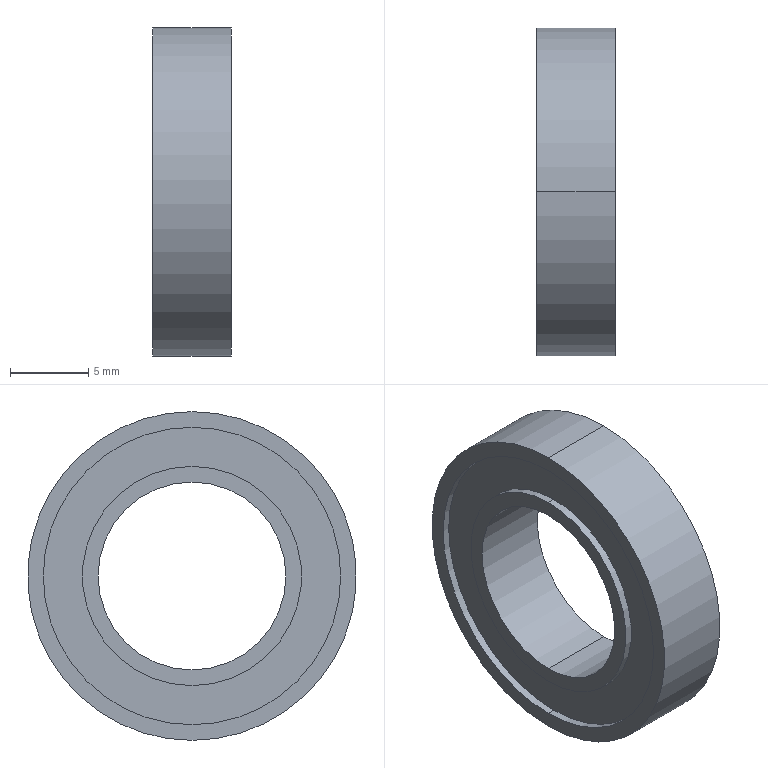Part | STEP file | Guide wheel mechanism revised.sldasm-Part-352 | 1 solid | 18 faces | box 5 x 21 x 21 mm | volume 1037 mm3 | cylinder 12 | plane 6 | commonest cylinder face diameters 14 x4 19 x4 12 x2 21 x2
STEP:
#1=CARTESIAN_POINT('',(5.,0.,7.));
#2=VERTEX_POINT('',#1);
#3=CARTESIAN_POINT('',(5.,0.,-7.));
#4=VERTEX_POINT('',#3);
#5=CARTESIAN_POINT('',(5.,0.,0.));
#6=DIRECTION('',(-1.,0.,0.));
#7=DIRECTION('',(0.,0.,1.));
#8=AXIS2_PLACEMENT_3D('',#5,#6,#7);
#9=CIRCLE('',#8,7.);
#10=EDGE_CURVE('',#2,#4,#9,.T.);
#11=ORIENTED_EDGE('',*,*,#10,.T.);
#12=CARTESIAN_POINT('',(4.5,0.,-7.));
#13=VERTEX_POINT('',#12);
#14=CARTESIAN_POINT('',(0.,0.,-7.));
#15=DIRECTION('',(-1.,0.,0.));
#16=VECTOR('',#15,1000.);
#17=LINE('',#14,#16);
#18=EDGE_CURVE('',#4,#13,#17,.T.);
#19=ORIENTED_EDGE('',*,*,#18,.T.);
#20=CARTESIAN_POINT('',(4.5,0.,7.));
#21=VERTEX_POINT('',#20);
#22=CARTESIAN_POINT('',(4.5,0.,0.));
#23=DIRECTION('',(-1.,0.,0.));
#24=DIRECTION('',(0.,0.,1.));
#25=AXIS2_PLACEMENT_3D('',#22,#23,#24);
#26=CIRCLE('',#25,7.);
#27=EDGE_CURVE('',#21,#13,#26,.T.);
#28=ORIENTED_EDGE('',*,*,#27,.F.);
#29=CARTESIAN_POINT('',(0.,0.,7.));
#30=DIRECTION('',(-1.,0.,0.));
#31=VECTOR('',#30,1000.);
#32=LINE('',#29,#31);
#33=EDGE_CURVE('',#2,#21,#32,.T.);
#34=ORIENTED_EDGE('',*,*,#33,.F.);
#35=EDGE_LOOP('',(#11,#19,#28,#34));
#36=FACE_OUTER_BOUND('',#35,.T.);
#37=CARTESIAN_POINT('',(0.,0.,0.));
#38=DIRECTION('',(-1.,0.,0.));
#39=DIRECTION('',(0.,0.,1.));
#40=AXIS2_PLACEMENT_3D('',#37,#38,#39);
#41=CYLINDRICAL_SURFACE('',#40,7.);
#42=ADVANCED_FACE('',(#36),#41,.T.);
#43=CARTESIAN_POINT('',(5.,0.,-9.5));
#44=VERTEX_POINT('',#43);
#45=CARTESIAN_POINT('',(5.,0.,9.5));
#46=VERTEX_POINT('',#45);
#47=CARTESIAN_POINT('',(5.,0.,0.));
#48=DIRECTION('',(-1.,0.,0.));
#49=DIRECTION('',(0.,0.,1.));
#50=AXIS2_PLACEMENT_3D('',#47,#48,#49);
#51=CIRCLE('',#50,9.5);
#52=EDGE_CURVE('',#44,#46,#51,.T.);
#53=ORIENTED_EDGE('',*,*,#52,.F.);
#54=CARTESIAN_POINT('',(4.5,0.,-9.5));
#55=VERTEX_POINT('',#54);
#56=CARTESIAN_POINT('',(0.,0.,-9.5));
#57=DIRECTION('',(-1.,0.,0.));
#58=VECTOR('',#57,1000.);
#59=LINE('',#56,#58);
#60=EDGE_CURVE('',#44,#55,#59,.T.);
#61=ORIENTED_EDGE('',*,*,#60,.T.);
#62=CARTESIAN_POINT('',(4.5,0.,9.5));
#63=VERTEX_POINT('',#62);
#64=CARTESIAN_POINT('',(4.5,0.,0.));
#65=DIRECTION('',(-1.,0.,0.));
#66=DIRECTION('',(0.,0.,1.));
#67=AXIS2_PLACEMENT_3D('',#64,#65,#66);
#68=CIRCLE('',#67,9.5);
#69=EDGE_CURVE('',#55,#63,#68,.T.);
#70=ORIENTED_EDGE('',*,*,#69,.T.);
#71=CARTESIAN_POINT('',(0.,0.,9.5));
#72=DIRECTION('',(-1.,0.,0.));
#73=VECTOR('',#72,1000.);
#74=LINE('',#71,#73);
#75=EDGE_CURVE('',#46,#63,#74,.T.);
#76=ORIENTED_EDGE('',*,*,#75,.F.);
#77=EDGE_LOOP('',(#53,#61,#70,#76));
#78=FACE_OUTER_BOUND('',#77,.T.);
#79=CARTESIAN_POINT('',(0.,0.,0.));
#80=DIRECTION('',(-1.,0.,0.));
#81=DIRECTION('',(0.,0.,1.));
#82=AXIS2_PLACEMENT_3D('',#79,#80,#81);
#83=CYLINDRICAL_SURFACE('',#82,9.5);
#84=ADVANCED_FACE('',(#78),#83,.F.);
#85=CARTESIAN_POINT('',(5.,0.,10.5));
#86=VERTEX_POINT('',#85);
#87=CARTESIAN_POINT('',(5.,0.,-10.5));
#88=VERTEX_POINT('',#87);
#89=CARTESIAN_POINT('',(5.,0.,0.));
#90=DIRECTION('',(-1.,0.,0.));
#91=DIRECTION('',(0.,0.,1.));
#92=AXIS2_PLACEMENT_3D('',#89,#90,#91);
#93=CIRCLE('',#92,10.5);
#94=EDGE_CURVE('',#86,#88,#93,.T.);
#95=ORIENTED_EDGE('',*,*,#94,.T.);
#96=CARTESIAN_POINT('',(0.,0.,-10.5));
#97=VERTEX_POINT('',#96);
#98=CARTESIAN_POINT('',(0.,0.,-10.5));
#99=DIRECTION('',(-1.,0.,0.));
#100=VECTOR('',#99,1000.);
#101=LINE('',#98,#100);
#102=EDGE_CURVE('',#88,#97,#101,.T.);
#103=ORIENTED_EDGE('',*,*,#102,.T.);
#104=CARTESIAN_POINT('',(0.,0.,10.5));
#105=VERTEX_POINT('',#104);
#106=CARTESIAN_POINT('',(0.,0.,0.));
#107=DIRECTION('',(-1.,0.,0.));
#108=DIRECTION('',(0.,0.,1.));
#109=AXIS2_PLACEMENT_3D('',#106,#107,#108);
#110=CIRCLE('',#109,10.5);
#111=EDGE_CURVE('',#105,#97,#110,.T.);
#112=ORIENTED_EDGE('',*,*,#111,.F.);
#113=CARTESIAN_POINT('',(0.,0.,10.5));
#114=DIRECTION('',(-1.,0.,0.));
#115=VECTOR('',#114,1000.);
#116=LINE('',#113,#115);
#117=EDGE_CURVE('',#86,#105,#116,.T.);
#118=ORIENTED_EDGE('',*,*,#117,.F.);
#119=EDGE_LOOP('',(#95,#103,#112,#118));
#120=FACE_OUTER_BOUND('',#119,.T.);
#121=CARTESIAN_POINT('',(0.,0.,0.));
#122=DIRECTION('',(-1.,0.,0.));
#123=DIRECTION('',(0.,0.,1.));
#124=AXIS2_PLACEMENT_3D('',#121,#122,#123);
#125=CYLINDRICAL_SURFACE('',#124,10.5);
#126=ADVANCED_FACE('',(#120),#125,.T.);
#127=CARTESIAN_POINT('',(0.5,0.,-9.5));
#128=VERTEX_POINT('',#127);
#129=CARTESIAN_POINT('',(0.5,0.,9.5));
#130=VERTEX_POINT('',#129);
#131=CARTESIAN_POINT('',(0.5,0.,0.));
#132=DIRECTION('',(-1.,0.,0.));
#133=DIRECTION('',(0.,0.,1.));
#134=AXIS2_PLACEMENT_3D('',#131,#132,#133);
#135=CIRCLE('',#134,9.5);
#136=EDGE_CURVE('',#128,#130,#135,.T.);
#137=ORIENTED_EDGE('',*,*,#136,.F.);
#138=CARTESIAN_POINT('',(0.,0.,-9.5));
#139=VERTEX_POINT('',#138);
#140=CARTESIAN_POINT('',(0.,0.,-9.5));
#141=DIRECTION('',(-1.,0.,0.));
#142=VECTOR('',#141,1000.);
#143=LINE('',#140,#142);
#144=EDGE_CURVE('',#128,#139,#143,.T.);
#145=ORIENTED_EDGE('',*,*,#144,.T.);
#146=CARTESIAN_POINT('',(0.,0.,9.5));
#147=VERTEX_POINT('',#146);
#148=CARTESIAN_POINT('',(0.,0.,0.));
#149=DIRECTION('',(-1.,0.,0.));
#150=DIRECTION('',(0.,0.,1.));
#151=AXIS2_PLACEMENT_3D('',#148,#149,#150);
#152=CIRCLE('',#151,9.5);
#153=EDGE_CURVE('',#139,#147,#152,.T.);
#154=ORIENTED_EDGE('',*,*,#153,.T.);
#155=CARTESIAN_POINT('',(0.,0.,9.5));
#156=DIRECTION('',(-1.,0.,0.));
#157=VECTOR('',#156,1000.);
#158=LINE('',#155,#157);
#159=EDGE_CURVE('',#130,#147,#158,.T.);
#160=ORIENTED_EDGE('',*,*,#159,.F.);
#161=EDGE_LOOP('',(#137,#145,#154,#160));
#162=FACE_OUTER_BOUND('',#161,.T.);
#163=CARTESIAN_POINT('',(0.,0.,0.));
#164=DIRECTION('',(-1.,0.,0.));
#165=DIRECTION('',(0.,0.,1.));
#166=AXIS2_PLACEMENT_3D('',#163,#164,#165);
#167=CYLINDRICAL_SURFACE('',#166,9.5);
#168=ADVANCED_FACE('',(#162),#167,.F.);
#169=CARTESIAN_POINT('',(0.5,0.,7.));
#170=VERTEX_POINT('',#169);
#171=CARTESIAN_POINT('',(0.5,0.,-7.));
#172=VERTEX_POINT('',#171);
#173=CARTESIAN_POINT('',(0.5,0.,0.));
#174=DIRECTION('',(-1.,0.,0.));
#175=DIRECTION('',(0.,0.,1.));
#176=AXIS2_PLACEMENT_3D('',#173,#174,#175);
#177=CIRCLE('',#176,7.);
#178=EDGE_CURVE('',#170,#172,#177,.T.);
#179=ORIENTED_EDGE('',*,*,#178,.T.);
#180=CARTESIAN_POINT('',(0.,0.,-7.));
#181=VERTEX_POINT('',#180);
#182=CARTESIAN_POINT('',(0.,0.,-7.));
#183=DIRECTION('',(-1.,0.,0.));
#184=VECTOR('',#183,1000.);
#185=LINE('',#182,#184);
#186=EDGE_CURVE('',#172,#181,#185,.T.);
#187=ORIENTED_EDGE('',*,*,#186,.T.);
#188=CARTESIAN_POINT('',(0.,0.,7.));
#189=VERTEX_POINT('',#188);
#190=CARTESIAN_POINT('',(0.,0.,0.));
#191=DIRECTION('',(-1.,0.,0.));
#192=DIRECTION('',(0.,0.,1.));
#193=AXIS2_PLACEMENT_3D('',#190,#191,#192);
#194=CIRCLE('',#193,7.);
#195=EDGE_CURVE('',#189,#181,#194,.T.);
#196=ORIENTED_EDGE('',*,*,#195,.F.);
#197=CARTESIAN_POINT('',(0.,0.,7.));
#198=DIRECTION('',(-1.,0.,0.));
#199=VECTOR('',#198,1000.);
#200=LINE('',#197,#199);
#201=EDGE_CURVE('',#170,#189,#200,.T.);
#202=ORIENTED_EDGE('',*,*,#201,.F.);
#203=EDGE_LOOP('',(#179,#187,#196,#202));
#204=FACE_OUTER_BOUND('',#203,.T.);
#205=CARTESIAN_POINT('',(0.,0.,0.));
#206=DIRECTION('',(-1.,0.,0.));
#207=DIRECTION('',(0.,0.,1.));
#208=AXIS2_PLACEMENT_3D('',#205,#206,#207);
#209=CYLINDRICAL_SURFACE('',#208,7.);
#210=ADVANCED_FACE('',(#204),#209,.T.);
#211=CARTESIAN_POINT('',(5.,0.,-6.));
#212=VERTEX_POINT('',#211);
#213=CARTESIAN_POINT('',(5.,0.,6.));
#214=VERTEX_POINT('',#213);
#215=CARTESIAN_POINT('',(5.,0.,0.));
#216=DIRECTION('',(-1.,0.,0.));
#217=DIRECTION('',(0.,0.,1.));
#218=AXIS2_PLACEMENT_3D('',#215,#216,#217);
#219=CIRCLE('',#218,6.);
#220=EDGE_CURVE('',#212,#214,#219,.T.);
#221=ORIENTED_EDGE('',*,*,#220,.F.);
#222=CARTESIAN_POINT('',(0.,0.,-6.));
#223=VERTEX_POINT('',#222);
#224=CARTESIAN_POINT('',(0.,0.,-6.));
#225=DIRECTION('',(-1.,0.,0.));
#226=VECTOR('',#225,1000.);
#227=LINE('',#224,#226);
#228=EDGE_CURVE('',#212,#223,#227,.T.);
#229=ORIENTED_EDGE('',*,*,#228,.T.);
#230=CARTESIAN_POINT('',(0.,0.,6.));
#231=VERTEX_POINT('',#230);
#232=CARTESIAN_POINT('',(0.,0.,0.));
#233=DIRECTION('',(-1.,0.,0.));
#234=DIRECTION('',(0.,0.,1.));
#235=AXIS2_PLACEMENT_3D('',#232,#233,#234);
#236=CIRCLE('',#235,6.);
#237=EDGE_CURVE('',#223,#231,#236,.T.);
#238=ORIENTED_EDGE('',*,*,#237,.T.);
#239=CARTESIAN_POINT('',(0.,0.,6.));
#240=DIRECTION('',(-1.,0.,0.));
#241=VECTOR('',#240,1000.);
#242=LINE('',#239,#241);
#243=EDGE_CURVE('',#214,#231,#242,.T.);
#244=ORIENTED_EDGE('',*,*,#243,.F.);
#245=EDGE_LOOP('',(#221,#229,#238,#244));
#246=FACE_OUTER_BOUND('',#245,.T.);
#247=CARTESIAN_POINT('',(0.,0.,0.));
#248=DIRECTION('',(-1.,0.,0.));
#249=DIRECTION('',(0.,0.,1.));
#250=AXIS2_PLACEMENT_3D('',#247,#248,#249);
#251=CYLINDRICAL_SURFACE('',#250,6.);
#252=ADVANCED_FACE('',(#246),#251,.F.);
#253=ORIENTED_EDGE('',*,*,#228,.F.);
#254=CARTESIAN_POINT('',(5.,0.,0.));
#255=DIRECTION('',(-1.,0.,0.));
#256=DIRECTION('',(0.,0.,1.));
#257=AXIS2_PLACEMENT_3D('',#254,#255,#256);
#258=CIRCLE('',#257,6.);
#259=EDGE_CURVE('',#214,#212,#258,.T.);
#260=ORIENTED_EDGE('',*,*,#259,.F.);
#261=ORIENTED_EDGE('',*,*,#243,.T.);
#262=CARTESIAN_POINT('',(0.,0.,0.));
#263=DIRECTION('',(-1.,0.,0.));
#264=DIRECTION('',(0.,0.,1.));
#265=AXIS2_PLACEMENT_3D('',#262,#263,#264);
#266=CIRCLE('',#265,6.);
#267=EDGE_CURVE('',#231,#223,#266,.T.);
#268=ORIENTED_EDGE('',*,*,#267,.T.);
#269=EDGE_LOOP('',(#253,#260,#261,#268));
#270=FACE_OUTER_BOUND('',#269,.T.);
#271=CARTESIAN_POINT('',(0.,0.,0.));
#272=DIRECTION('',(-1.,0.,0.));
#273=DIRECTION('',(0.,0.,1.));
#274=AXIS2_PLACEMENT_3D('',#271,#272,#273);
#275=CYLINDRICAL_SURFACE('',#274,6.);
#276=ADVANCED_FACE('',(#270),#275,.F.);
#277=ORIENTED_EDGE('',*,*,#267,.F.);
#278=ORIENTED_EDGE('',*,*,#237,.F.);
#279=EDGE_LOOP('',(#277,#278));
#280=FACE_BOUND('',#279,.T.);
#281=ORIENTED_EDGE('',*,*,#195,.T.);
#282=CARTESIAN_POINT('',(0.,0.,0.));
#283=DIRECTION('',(-1.,0.,0.));
#284=DIRECTION('',(0.,0.,1.));
#285=AXIS2_PLACEMENT_3D('',#282,#283,#284);
#286=CIRCLE('',#285,7.);
#287=EDGE_CURVE('',#181,#189,#286,.T.);
#288=ORIENTED_EDGE('',*,*,#287,.T.);
#289=EDGE_LOOP('',(#281,#288));
#290=FACE_OUTER_BOUND('',#289,.T.);
#291=CARTESIAN_POINT('',(0.,6.,0.));
#292=DIRECTION('',(1.,0.,0.));
#293=DIRECTION('',(0.,0.,-1.));
#294=AXIS2_PLACEMENT_3D('',#291,#292,#293);
#295=PLANE('',#294);
#296=ADVANCED_FACE('',(#280,#290),#295,.F.);
#297=ORIENTED_EDGE('',*,*,#186,.F.);
#298=CARTESIAN_POINT('',(0.5,0.,0.));
#299=DIRECTION('',(-1.,0.,0.));
#300=DIRECTION('',(0.,0.,1.));
#301=AXIS2_PLACEMENT_3D('',#298,#299,#300);
#302=CIRCLE('',#301,7.);
#303=EDGE_CURVE('',#172,#170,#302,.T.);
#304=ORIENTED_EDGE('',*,*,#303,.T.);
#305=ORIENTED_EDGE('',*,*,#201,.T.);
#306=ORIENTED_EDGE('',*,*,#287,.F.);
#307=EDGE_LOOP('',(#297,#304,#305,#306));
#308=FACE_OUTER_BOUND('',#307,.T.);
#309=CARTESIAN_POINT('',(0.,0.,0.));
#310=DIRECTION('',(-1.,0.,0.));
#311=DIRECTION('',(0.,0.,1.));
#312=AXIS2_PLACEMENT_3D('',#309,#310,#311);
#313=CYLINDRICAL_SURFACE('',#312,7.);
#314=ADVANCED_FACE('',(#308),#313,.T.);
#315=ORIENTED_EDGE('',*,*,#178,.F.);
#316=ORIENTED_EDGE('',*,*,#303,.F.);
#317=EDGE_LOOP('',(#315,#316));
#318=FACE_BOUND('',#317,.T.);
#319=CARTESIAN_POINT('',(0.5,0.,0.));
#320=DIRECTION('',(-1.,0.,0.));
#321=DIRECTION('',(0.,0.,1.));
#322=AXIS2_PLACEMENT_3D('',#319,#320,#321);
#323=CIRCLE('',#322,9.5);
#324=EDGE_CURVE('',#130,#128,#323,.T.);
#325=ORIENTED_EDGE('',*,*,#324,.T.);
#326=ORIENTED_EDGE('',*,*,#136,.T.);
#327=EDGE_LOOP('',(#325,#326));
#328=FACE_OUTER_BOUND('',#327,.T.);
#329=CARTESIAN_POINT('',(0.5,7.,0.));
#330=DIRECTION('',(1.,0.,0.));
#331=DIRECTION('',(0.,0.,-1.));
#332=AXIS2_PLACEMENT_3D('',#329,#330,#331);
#333=PLANE('',#332);
#334=ADVANCED_FACE('',(#318,#328),#333,.F.);
#335=ORIENTED_EDGE('',*,*,#144,.F.);
#336=ORIENTED_EDGE('',*,*,#324,.F.);
#337=ORIENTED_EDGE('',*,*,#159,.T.);
#338=CARTESIAN_POINT('',(0.,0.,0.));
#339=DIRECTION('',(-1.,0.,0.));
#340=DIRECTION('',(0.,0.,1.));
#341=AXIS2_PLACEMENT_3D('',#338,#339,#340);
#342=CIRCLE('',#341,9.5);
#343=EDGE_CURVE('',#147,#139,#342,.T.);
#344=ORIENTED_EDGE('',*,*,#343,.T.);
#345=EDGE_LOOP('',(#335,#336,#337,#344));
#346=FACE_OUTER_BOUND('',#345,.T.);
#347=CARTESIAN_POINT('',(0.,0.,0.));
#348=DIRECTION('',(-1.,0.,0.));
#349=DIRECTION('',(0.,0.,1.));
#350=AXIS2_PLACEMENT_3D('',#347,#348,#349);
#351=CYLINDRICAL_SURFACE('',#350,9.5);
#352=ADVANCED_FACE('',(#346),#351,.F.);
#353=ORIENTED_EDGE('',*,*,#343,.F.);
#354=ORIENTED_EDGE('',*,*,#153,.F.);
#355=EDGE_LOOP('',(#353,#354));
#356=FACE_BOUND('',#355,.T.);
#357=ORIENTED_EDGE('',*,*,#111,.T.);
#358=CARTESIAN_POINT('',(0.,0.,0.));
#359=DIRECTION('',(-1.,0.,0.));
#360=DIRECTION('',(0.,0.,1.));
#361=AXIS2_PLACEMENT_3D('',#358,#359,#360);
#362=CIRCLE('',#361,10.5);
#363=EDGE_CURVE('',#97,#105,#362,.T.);
#364=ORIENTED_EDGE('',*,*,#363,.T.);
#365=EDGE_LOOP('',(#357,#364));
#366=FACE_OUTER_BOUND('',#365,.T.);
#367=CARTESIAN_POINT('',(0.,9.5,0.));
#368=DIRECTION('',(1.,0.,0.));
#369=DIRECTION('',(0.,0.,-1.));
#370=AXIS2_PLACEMENT_3D('',#367,#368,#369);
#371=PLANE('',#370);
#372=ADVANCED_FACE('',(#356,#366),#371,.F.);
#373=ORIENTED_EDGE('',*,*,#102,.F.);
#374=CARTESIAN_POINT('',(5.,0.,0.));
#375=DIRECTION('',(-1.,0.,0.));
#376=DIRECTION('',(0.,0.,1.));
#377=AXIS2_PLACEMENT_3D('',#374,#375,#376);
#378=CIRCLE('',#377,10.5);
#379=EDGE_CURVE('',#88,#86,#378,.T.);
#380=ORIENTED_EDGE('',*,*,#379,.T.);
#381=ORIENTED_EDGE('',*,*,#117,.T.);
#382=ORIENTED_EDGE('',*,*,#363,.F.);
#383=EDGE_LOOP('',(#373,#380,#381,#382));
#384=FACE_OUTER_BOUND('',#383,.T.);
#385=CARTESIAN_POINT('',(0.,0.,0.));
#386=DIRECTION('',(-1.,0.,0.));
#387=DIRECTION('',(0.,0.,1.));
#388=AXIS2_PLACEMENT_3D('',#385,#386,#387);
#389=CYLINDRICAL_SURFACE('',#388,10.5);
#390=ADVANCED_FACE('',(#384),#389,.T.);
#391=ORIENTED_EDGE('',*,*,#94,.F.);
#392=ORIENTED_EDGE('',*,*,#379,.F.);
#393=EDGE_LOOP('',(#391,#392));
#394=FACE_OUTER_BOUND('',#393,.T.);
#395=CARTESIAN_POINT('',(5.,0.,0.));
#396=DIRECTION('',(-1.,0.,0.));
#397=DIRECTION('',(0.,0.,1.));
#398=AXIS2_PLACEMENT_3D('',#395,#396,#397);
#399=CIRCLE('',#398,9.5);
#400=EDGE_CURVE('',#46,#44,#399,.T.);
#401=ORIENTED_EDGE('',*,*,#400,.T.);
#402=ORIENTED_EDGE('',*,*,#52,.T.);
#403=EDGE_LOOP('',(#401,#402));
#404=FACE_BOUND('',#403,.T.);
#405=CARTESIAN_POINT('',(5.,10.5,0.));
#406=DIRECTION('',(-1.,0.,0.));
#407=DIRECTION('',(0.,0.,1.));
#408=AXIS2_PLACEMENT_3D('',#405,#406,#407);
#409=PLANE('',#408);
#410=ADVANCED_FACE('',(#394,#404),#409,.F.);
#411=ORIENTED_EDGE('',*,*,#60,.F.);
#412=ORIENTED_EDGE('',*,*,#400,.F.);
#413=ORIENTED_EDGE('',*,*,#75,.T.);
#414=CARTESIAN_POINT('',(4.5,0.,0.));
#415=DIRECTION('',(-1.,0.,0.));
#416=DIRECTION('',(0.,0.,1.));
#417=AXIS2_PLACEMENT_3D('',#414,#415,#416);
#418=CIRCLE('',#417,9.5);
#419=EDGE_CURVE('',#63,#55,#418,.T.);
#420=ORIENTED_EDGE('',*,*,#419,.T.);
#421=EDGE_LOOP('',(#411,#412,#413,#420));
#422=FACE_OUTER_BOUND('',#421,.T.);
#423=CARTESIAN_POINT('',(0.,0.,0.));
#424=DIRECTION('',(-1.,0.,0.));
#425=DIRECTION('',(0.,0.,1.));
#426=AXIS2_PLACEMENT_3D('',#423,#424,#425);
#427=CYLINDRICAL_SURFACE('',#426,9.5);
#428=ADVANCED_FACE('',(#422),#427,.F.);
#429=ORIENTED_EDGE('',*,*,#419,.F.);
#430=ORIENTED_EDGE('',*,*,#69,.F.);
#431=EDGE_LOOP('',(#429,#430));
#432=FACE_OUTER_BOUND('',#431,.T.);
#433=ORIENTED_EDGE('',*,*,#27,.T.);
#434=CARTESIAN_POINT('',(4.5,0.,0.));
#435=DIRECTION('',(-1.,0.,0.));
#436=DIRECTION('',(0.,0.,1.));
#437=AXIS2_PLACEMENT_3D('',#434,#435,#436);
#438=CIRCLE('',#437,7.);
#439=EDGE_CURVE('',#13,#21,#438,.T.);
#440=ORIENTED_EDGE('',*,*,#439,.T.);
#441=EDGE_LOOP('',(#433,#440));
#442=FACE_BOUND('',#441,.T.);
#443=CARTESIAN_POINT('',(4.5,9.5,0.));
#444=DIRECTION('',(-1.,0.,0.));
#445=DIRECTION('',(0.,0.,1.));
#446=AXIS2_PLACEMENT_3D('',#443,#444,#445);
#447=PLANE('',#446);
#448=ADVANCED_FACE('',(#432,#442),#447,.F.);
#449=ORIENTED_EDGE('',*,*,#18,.F.);
#450=CARTESIAN_POINT('',(5.,0.,0.));
#451=DIRECTION('',(-1.,0.,0.));
#452=DIRECTION('',(0.,0.,1.));
#453=AXIS2_PLACEMENT_3D('',#450,#451,#452);
#454=CIRCLE('',#453,7.);
#455=EDGE_CURVE('',#4,#2,#454,.T.);
#456=ORIENTED_EDGE('',*,*,#455,.T.);
#457=ORIENTED_EDGE('',*,*,#33,.T.);
#458=ORIENTED_EDGE('',*,*,#439,.F.);
#459=EDGE_LOOP('',(#449,#456,#457,#458));
#460=FACE_OUTER_BOUND('',#459,.T.);
#461=CARTESIAN_POINT('',(0.,0.,0.));
#462=DIRECTION('',(-1.,0.,0.));
#463=DIRECTION('',(0.,0.,1.));
#464=AXIS2_PLACEMENT_3D('',#461,#462,#463);
#465=CYLINDRICAL_SURFACE('',#464,7.);
#466=ADVANCED_FACE('',(#460),#465,.T.);
#467=ORIENTED_EDGE('',*,*,#10,.F.);
#468=ORIENTED_EDGE('',*,*,#455,.F.);
#469=EDGE_LOOP('',(#467,#468));
#470=FACE_OUTER_BOUND('',#469,.T.);
#471=ORIENTED_EDGE('',*,*,#259,.T.);
#472=ORIENTED_EDGE('',*,*,#220,.T.);
#473=EDGE_LOOP('',(#471,#472));
#474=FACE_BOUND('',#473,.T.);
#475=CARTESIAN_POINT('',(5.,7.,0.));
#476=DIRECTION('',(-1.,0.,0.));
#477=DIRECTION('',(0.,0.,1.));
#478=AXIS2_PLACEMENT_3D('',#475,#476,#477);
#479=PLANE('',#478);
#480=ADVANCED_FACE('',(#470,#474),#479,.F.);
#481=CLOSED_SHELL('',(#42,#84,#126,#168,#210,#252,#276,#296,#314,#334,#352,#372,#390,#410,#428,#448,#466,#480));
#482=MANIFOLD_SOLID_BREP('',#481);
#483=CARTESIAN_POINT('',(0.,0.,0.));
#484=DIRECTION('',(0.,0.,1.));
#485=DIRECTION('',(1.,0.,0.));
#486=AXIS2_PLACEMENT_3D('',#483,#484,#485);
#487=(LENGTH_UNIT()NAMED_UNIT(*)SI_UNIT(.MILLI.,.METRE.));
#488=UNCERTAINTY_MEASURE_WITH_UNIT(LENGTH_MEASURE(0.00001),#487,'','');
#489=(NAMED_UNIT(*)PLANE_ANGLE_UNIT()SI_UNIT($,.RADIAN.));
#490=(NAMED_UNIT(*)SI_UNIT($,.STERADIAN.)SOLID_ANGLE_UNIT());
#491=(GEOMETRIC_REPRESENTATION_CONTEXT(3)GLOBAL_UNCERTAINTY_ASSIGNED_CONTEXT((#488))GLOBAL_UNIT_ASSIGNED_CONTEXT((#487,#489,#490))REPRESENTATION_CONTEXT('',''));
#492=ADVANCED_BREP_SHAPE_REPRESENTATION('',(#482,#486),#491);